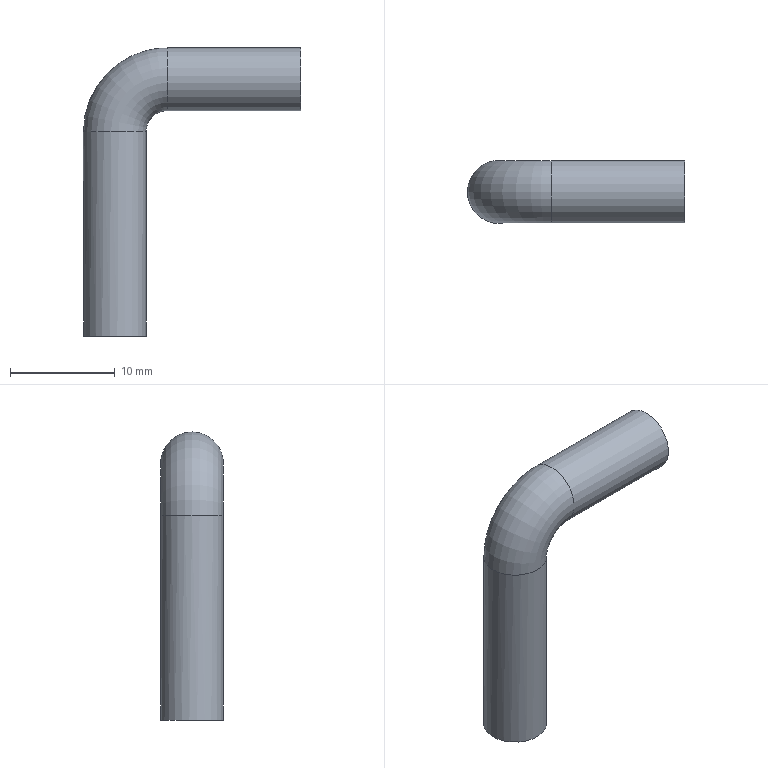Part | STEP file | lll_id4350_x_t | 1 solid | 8 faces | box 20.765 x 6 x 27.556 mm | volume 1010 mm3 | cylinder 4 | torus 2 | plane 2 | commonest cylinder face diameters 2 x2 6 x2
STEP:
#1=CARTESIAN_POINT('',(686.259,-421.593,-14.));
#2=VERTEX_POINT('',#1);
#3=CARTESIAN_POINT('',(686.259,-421.593,-13.));
#4=DIRECTION('',(-1.,0.,0.));
#5=DIRECTION('',(0.,0.,-1.));
#6=AXIS2_PLACEMENT_3D('',#3,#4,#5);
#7=CIRCLE('',#6,1.);
#8=EDGE_CURVE('',#2,#2,#7,.T.);
#9=ORIENTED_EDGE('',*,*,#8,.T.);
#10=EDGE_LOOP('',(#9));
#11=FACE_BOUND('',#10,.T.);
#12=CARTESIAN_POINT('',(699.024,-421.593,-14.));
#13=VERTEX_POINT('',#12);
#14=CARTESIAN_POINT('',(699.024,-421.593,-13.));
#15=DIRECTION('',(-1.,0.,0.));
#16=DIRECTION('',(0.,0.,-1.));
#17=AXIS2_PLACEMENT_3D('',#14,#15,#16);
#18=CIRCLE('',#17,1.);
#19=EDGE_CURVE('',#13,#13,#18,.T.);
#20=ORIENTED_EDGE('',*,*,#19,.F.);
#21=EDGE_LOOP('',(#20));
#22=FACE_BOUND('',#21,.T.);
#23=CARTESIAN_POINT('',(686.259,-421.593,-13.));
#24=DIRECTION('',(1.,0.,0.));
#25=DIRECTION('',(0.,0.,1.));
#26=AXIS2_PLACEMENT_3D('',#23,#24,#25);
#27=CYLINDRICAL_SURFACE('',#26,1.);
#28=ADVANCED_FACE('',(#11,#22),#27,.F.);
#29=CARTESIAN_POINT('',(682.259,-421.593,-18.));
#30=VERTEX_POINT('',#29);
#31=CARTESIAN_POINT('',(681.259,-421.593,-18.));
#32=DIRECTION('',(0.,0.,-1.));
#33=DIRECTION('',(1.,0.,0.));
#34=AXIS2_PLACEMENT_3D('',#31,#32,#33);
#35=CIRCLE('',#34,1.);
#36=EDGE_CURVE('',#30,#30,#35,.T.);
#37=ORIENTED_EDGE('',*,*,#36,.T.);
#38=EDGE_LOOP('',(#37));
#39=FACE_BOUND('',#38,.T.);
#40=ORIENTED_EDGE('',*,*,#8,.F.);
#41=EDGE_LOOP('',(#40));
#42=FACE_BOUND('',#41,.T.);
#43=CARTESIAN_POINT('',(686.259,-421.593,-18.));
#44=DIRECTION('',(0.,1.,0.));
#45=DIRECTION('',(0.,0.,1.));
#46=AXIS2_PLACEMENT_3D('',#43,#44,#45);
#47=TOROIDAL_SURFACE('',#46,5.,1.);
#48=ADVANCED_FACE('',(#39,#42),#47,.F.);
#49=ORIENTED_EDGE('',*,*,#36,.F.);
#50=EDGE_LOOP('',(#49));
#51=FACE_BOUND('',#50,.T.);
#52=CARTESIAN_POINT('',(681.259,-420.593,-37.556));
#53=VERTEX_POINT('',#52);
#54=CARTESIAN_POINT('',(681.259,-421.593,-37.556));
#55=DIRECTION('',(0.,0.,-1.));
#56=DIRECTION('',(0.,1.,0.));
#57=AXIS2_PLACEMENT_3D('',#54,#55,#56);
#58=CIRCLE('',#57,1.);
#59=EDGE_CURVE('',#53,#53,#58,.T.);
#60=ORIENTED_EDGE('',*,*,#59,.T.);
#61=EDGE_LOOP('',(#60));
#62=FACE_BOUND('',#61,.T.);
#63=CARTESIAN_POINT('',(681.259,-421.593,-135.5));
#64=DIRECTION('',(0.,0.,1.));
#65=DIRECTION('',(0.,-1.,0.));
#66=AXIS2_PLACEMENT_3D('',#63,#64,#65);
#67=CYLINDRICAL_SURFACE('',#66,1.);
#68=ADVANCED_FACE('',(#51,#62),#67,.F.);
#69=ORIENTED_EDGE('',*,*,#19,.T.);
#70=EDGE_LOOP('',(#69));
#71=FACE_BOUND('',#70,.T.);
#72=CARTESIAN_POINT('',(699.024,-421.593,-16.));
#73=VERTEX_POINT('',#72);
#74=CARTESIAN_POINT('',(699.024,-421.593,-13.));
#75=DIRECTION('',(-1.,0.,0.));
#76=DIRECTION('',(0.,0.,-1.));
#77=AXIS2_PLACEMENT_3D('',#74,#75,#76);
#78=CIRCLE('',#77,3.);
#79=EDGE_CURVE('',#73,#73,#78,.T.);
#80=ORIENTED_EDGE('',*,*,#79,.F.);
#81=EDGE_LOOP('',(#80));
#82=FACE_BOUND('',#81,.T.);
#83=CARTESIAN_POINT('',(699.024,-421.593,-13.));
#84=DIRECTION('',(1.,0.,0.));
#85=DIRECTION('',(0.,0.,-1.));
#86=AXIS2_PLACEMENT_3D('',#83,#84,#85);
#87=PLANE('',#86);
#88=ADVANCED_FACE('',(#71,#82),#87,.T.);
#89=CARTESIAN_POINT('',(686.259,-421.593,-16.));
#90=VERTEX_POINT('',#89);
#91=CARTESIAN_POINT('',(686.259,-421.593,-13.));
#92=DIRECTION('',(-1.,0.,0.));
#93=DIRECTION('',(0.,0.,-1.));
#94=AXIS2_PLACEMENT_3D('',#91,#92,#93);
#95=CIRCLE('',#94,3.);
#96=EDGE_CURVE('',#90,#90,#95,.T.);
#97=ORIENTED_EDGE('',*,*,#96,.F.);
#98=EDGE_LOOP('',(#97));
#99=FACE_BOUND('',#98,.T.);
#100=ORIENTED_EDGE('',*,*,#79,.T.);
#101=EDGE_LOOP('',(#100));
#102=FACE_BOUND('',#101,.T.);
#103=CARTESIAN_POINT('',(686.259,-421.593,-13.));
#104=DIRECTION('',(1.,0.,0.));
#105=DIRECTION('',(0.,0.,1.));
#106=AXIS2_PLACEMENT_3D('',#103,#104,#105);
#107=CYLINDRICAL_SURFACE('',#106,3.);
#108=ADVANCED_FACE('',(#99,#102),#107,.T.);
#109=CARTESIAN_POINT('',(684.259,-421.593,-18.));
#110=VERTEX_POINT('',#109);
#111=CARTESIAN_POINT('',(681.259,-421.593,-18.));
#112=DIRECTION('',(0.,0.,-1.));
#113=DIRECTION('',(1.,0.,0.));
#114=AXIS2_PLACEMENT_3D('',#111,#112,#113);
#115=CIRCLE('',#114,3.);
#116=EDGE_CURVE('',#110,#110,#115,.T.);
#117=ORIENTED_EDGE('',*,*,#116,.F.);
#118=EDGE_LOOP('',(#117));
#119=FACE_BOUND('',#118,.T.);
#120=ORIENTED_EDGE('',*,*,#96,.T.);
#121=EDGE_LOOP('',(#120));
#122=FACE_BOUND('',#121,.T.);
#123=CARTESIAN_POINT('',(686.259,-421.593,-18.));
#124=DIRECTION('',(0.,1.,0.));
#125=DIRECTION('',(0.,0.,1.));
#126=AXIS2_PLACEMENT_3D('',#123,#124,#125);
#127=TOROIDAL_SURFACE('',#126,5.,3.);
#128=ADVANCED_FACE('',(#119,#122),#127,.T.);
#129=ORIENTED_EDGE('',*,*,#116,.T.);
#130=EDGE_LOOP('',(#129));
#131=FACE_BOUND('',#130,.T.);
#132=CARTESIAN_POINT('',(681.259,-418.593,-37.556));
#133=VERTEX_POINT('',#132);
#134=CARTESIAN_POINT('',(681.259,-421.593,-37.556));
#135=DIRECTION('',(0.,0.,1.));
#136=DIRECTION('',(0.,1.,0.));
#137=AXIS2_PLACEMENT_3D('',#134,#135,#136);
#138=CIRCLE('',#137,3.);
#139=EDGE_CURVE('',#133,#133,#138,.T.);
#140=ORIENTED_EDGE('',*,*,#139,.T.);
#141=EDGE_LOOP('',(#140));
#142=FACE_BOUND('',#141,.T.);
#143=CARTESIAN_POINT('',(681.259,-421.593,-135.5));
#144=DIRECTION('',(0.,0.,1.));
#145=DIRECTION('',(0.,-1.,0.));
#146=AXIS2_PLACEMENT_3D('',#143,#144,#145);
#147=CYLINDRICAL_SURFACE('',#146,3.);
#148=ADVANCED_FACE('',(#131,#142),#147,.T.);
#149=ORIENTED_EDGE('',*,*,#139,.F.);
#150=EDGE_LOOP('',(#149));
#151=FACE_BOUND('',#150,.T.);
#152=ORIENTED_EDGE('',*,*,#59,.F.);
#153=EDGE_LOOP('',(#152));
#154=FACE_BOUND('',#153,.T.);
#155=CARTESIAN_POINT('',(618.161,4438.394,-37.556));
#156=DIRECTION('',(0.,0.,-1.));
#157=DIRECTION('',(0.,1.,0.));
#158=AXIS2_PLACEMENT_3D('',#155,#156,#157);
#159=PLANE('',#158);
#160=ADVANCED_FACE('',(#151,#154),#159,.T.);
#161=CLOSED_SHELL('',(#28,#48,#68,#88,#108,#128,#148,#160));
#162=MANIFOLD_SOLID_BREP('',#161);
#163=(LENGTH_UNIT()NAMED_UNIT(*)SI_UNIT(.MILLI.,.METRE.));
#164=UNCERTAINTY_MEASURE_WITH_UNIT(LENGTH_MEASURE(0.00002),#163,'','');
#165=(NAMED_UNIT(*)PLANE_ANGLE_UNIT()SI_UNIT($,.RADIAN.));
#166=PLANE_ANGLE_MEASURE_WITH_UNIT(PLANE_ANGLE_MEASURE(0.01745),#165);
#167=DIMENSIONAL_EXPONENTS(0.,0.,0.,0.,0.,0.,0.);
#168=(CONVERSION_BASED_UNIT('DEGREE',#166)NAMED_UNIT(#167)PLANE_ANGLE_UNIT());
#169=(NAMED_UNIT(*)SI_UNIT($,.STERADIAN.)SOLID_ANGLE_UNIT());
#170=(GEOMETRIC_REPRESENTATION_CONTEXT(3)GLOBAL_UNCERTAINTY_ASSIGNED_CONTEXT((#164))GLOBAL_UNIT_ASSIGNED_CONTEXT((#163,#168,#169))REPRESENTATION_CONTEXT('',''));
#171=ADVANCED_BREP_SHAPE_REPRESENTATION('',(#162),#170);